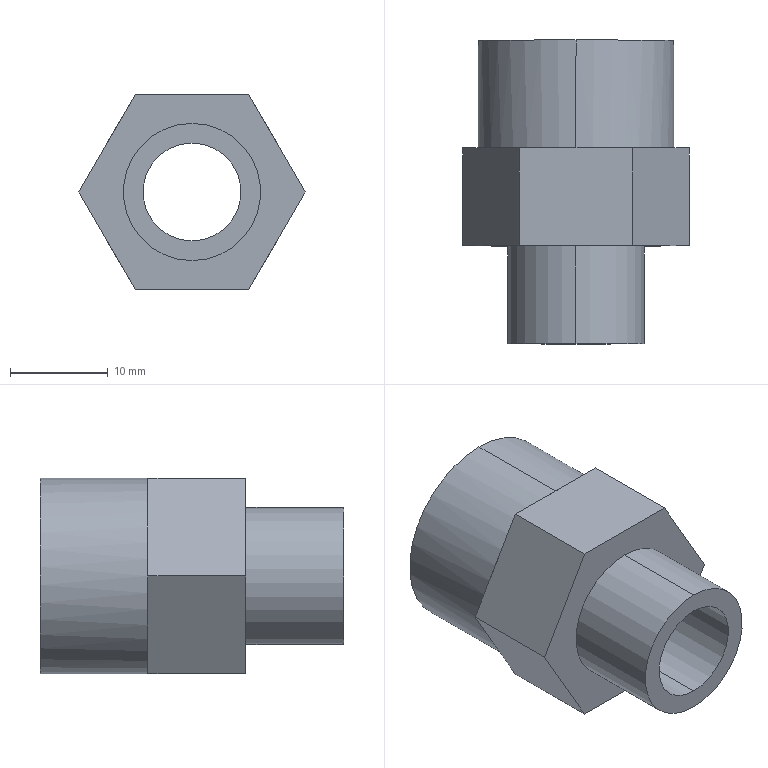Part | SolidWorks | features BossThin 1, ExtruThin 1, ICE 1 | 1 solid | 24 faces | box 23.094 x 31 x 20 mm | volume 4677 mm3 | plane 16 | cylinder 8 | commonest cylinder face diameters 10 x2 14 x2 16 x2 20 x2
STEP:
#1=CARTESIAN_POINT('',(0.,-20.,-7.));
#2=VERTEX_POINT('',#1);
#3=CARTESIAN_POINT('',(0.,-20.,7.));
#4=VERTEX_POINT('',#3);
#5=CARTESIAN_POINT('',(0.,-20.,0.));
#6=DIRECTION('',(0.,-1.,0.));
#7=DIRECTION('',(1.,0.,0.));
#8=AXIS2_PLACEMENT_3D('',#5,#6,#7);
#9=CIRCLE('',#8,7.);
#10=EDGE_CURVE('',#2,#4,#9,.T.);
#11=ORIENTED_EDGE('',*,*,#10,.F.);
#12=CARTESIAN_POINT('',(0.,-10.,-7.));
#13=VERTEX_POINT('',#12);
#14=CARTESIAN_POINT('',(0.,-20.,-7.));
#15=DIRECTION('',(0.,1.,0.));
#16=VECTOR('',#15,1000.);
#17=LINE('',#14,#16);
#18=EDGE_CURVE('',#2,#13,#17,.T.);
#19=ORIENTED_EDGE('',*,*,#18,.T.);
#20=CARTESIAN_POINT('',(0.,-10.,7.));
#21=VERTEX_POINT('',#20);
#22=CARTESIAN_POINT('',(0.,-10.,0.));
#23=DIRECTION('',(0.,-1.,0.));
#24=DIRECTION('',(1.,0.,0.));
#25=AXIS2_PLACEMENT_3D('',#22,#23,#24);
#26=CIRCLE('',#25,7.);
#27=EDGE_CURVE('',#13,#21,#26,.T.);
#28=ORIENTED_EDGE('',*,*,#27,.T.);
#29=CARTESIAN_POINT('',(0.,-20.,7.));
#30=DIRECTION('',(0.,1.,0.));
#31=VECTOR('',#30,1000.);
#32=LINE('',#29,#31);
#33=EDGE_CURVE('',#4,#21,#32,.T.);
#34=ORIENTED_EDGE('',*,*,#33,.F.);
#35=EDGE_LOOP('',(#11,#19,#28,#34));
#36=FACE_OUTER_BOUND('',#35,.T.);
#37=CARTESIAN_POINT('',(0.,-20.,0.));
#38=DIRECTION('',(0.,1.,0.));
#39=DIRECTION('',(0.,0.,1.));
#40=AXIS2_PLACEMENT_3D('',#37,#38,#39);
#41=CYLINDRICAL_SURFACE('',#40,7.);
#42=ADVANCED_FACE('',(#36),#41,.T.);
#43=CARTESIAN_POINT('',(0.,-20.,5.));
#44=VERTEX_POINT('',#43);
#45=CARTESIAN_POINT('',(0.,-20.,-5.));
#46=VERTEX_POINT('',#45);
#47=CARTESIAN_POINT('',(0.,-20.,0.));
#48=DIRECTION('',(0.,-1.,0.));
#49=DIRECTION('',(0.,0.,-1.));
#50=AXIS2_PLACEMENT_3D('',#47,#48,#49);
#51=CIRCLE('',#50,5.);
#52=EDGE_CURVE('',#44,#46,#51,.T.);
#53=ORIENTED_EDGE('',*,*,#52,.T.);
#54=CARTESIAN_POINT('',(0.,0.,-5.));
#55=VERTEX_POINT('',#54);
#56=CARTESIAN_POINT('',(0.,-10.,-5.));
#57=DIRECTION('',(0.,1.,0.));
#58=VECTOR('',#57,1000.);
#59=LINE('',#56,#58);
#60=EDGE_CURVE('',#46,#55,#59,.T.);
#61=ORIENTED_EDGE('',*,*,#60,.T.);
#62=CARTESIAN_POINT('',(0.,0.,5.));
#63=VERTEX_POINT('',#62);
#64=CARTESIAN_POINT('',(0.,0.,0.));
#65=DIRECTION('',(0.,-1.,0.));
#66=DIRECTION('',(0.,0.,-1.));
#67=AXIS2_PLACEMENT_3D('',#64,#65,#66);
#68=CIRCLE('',#67,5.);
#69=EDGE_CURVE('',#63,#55,#68,.T.);
#70=ORIENTED_EDGE('',*,*,#69,.F.);
#71=CARTESIAN_POINT('',(0.,-10.,5.));
#72=DIRECTION('',(0.,1.,0.));
#73=VECTOR('',#72,1000.);
#74=LINE('',#71,#73);
#75=EDGE_CURVE('',#44,#63,#74,.T.);
#76=ORIENTED_EDGE('',*,*,#75,.F.);
#77=EDGE_LOOP('',(#53,#61,#70,#76));
#78=FACE_OUTER_BOUND('',#77,.T.);
#79=CARTESIAN_POINT('',(0.,-10.,0.));
#80=DIRECTION('',(0.,1.,0.));
#81=DIRECTION('',(0.,0.,1.));
#82=AXIS2_PLACEMENT_3D('',#79,#80,#81);
#83=CYLINDRICAL_SURFACE('',#82,5.);
#84=ADVANCED_FACE('',(#78),#83,.F.);
#85=CARTESIAN_POINT('',(0.,11.,-8.));
#86=VERTEX_POINT('',#85);
#87=CARTESIAN_POINT('',(0.,11.,8.));
#88=VERTEX_POINT('',#87);
#89=CARTESIAN_POINT('',(0.,11.,0.));
#90=DIRECTION('',(0.,1.,0.));
#91=DIRECTION('',(1.,0.,0.));
#92=AXIS2_PLACEMENT_3D('',#89,#90,#91);
#93=CIRCLE('',#92,8.);
#94=EDGE_CURVE('',#86,#88,#93,.T.);
#95=ORIENTED_EDGE('',*,*,#94,.T.);
#96=CARTESIAN_POINT('',(0.,0.,8.));
#97=VERTEX_POINT('',#96);
#98=CARTESIAN_POINT('',(0.,11.,8.));
#99=DIRECTION('',(0.,-1.,0.));
#100=VECTOR('',#99,1000.);
#101=LINE('',#98,#100);
#102=EDGE_CURVE('',#88,#97,#101,.T.);
#103=ORIENTED_EDGE('',*,*,#102,.T.);
#104=CARTESIAN_POINT('',(0.,0.,-8.));
#105=VERTEX_POINT('',#104);
#106=CARTESIAN_POINT('',(0.,0.,0.));
#107=DIRECTION('',(0.,1.,0.));
#108=DIRECTION('',(1.,0.,0.));
#109=AXIS2_PLACEMENT_3D('',#106,#107,#108);
#110=CIRCLE('',#109,8.);
#111=EDGE_CURVE('',#105,#97,#110,.T.);
#112=ORIENTED_EDGE('',*,*,#111,.F.);
#113=CARTESIAN_POINT('',(0.,11.,-8.));
#114=DIRECTION('',(0.,-1.,0.));
#115=VECTOR('',#114,1000.);
#116=LINE('',#113,#115);
#117=EDGE_CURVE('',#86,#105,#116,.T.);
#118=ORIENTED_EDGE('',*,*,#117,.F.);
#119=EDGE_LOOP('',(#95,#103,#112,#118));
#120=FACE_OUTER_BOUND('',#119,.T.);
#121=CARTESIAN_POINT('',(0.,11.,0.));
#122=DIRECTION('',(0.,-1.,0.));
#123=DIRECTION('',(0.,0.,-1.));
#124=AXIS2_PLACEMENT_3D('',#121,#122,#123);
#125=CYLINDRICAL_SURFACE('',#124,8.);
#126=ADVANCED_FACE('',(#120),#125,.F.);
#127=CARTESIAN_POINT('',(0.,11.,10.));
#128=VERTEX_POINT('',#127);
#129=CARTESIAN_POINT('',(0.,11.,-10.));
#130=VERTEX_POINT('',#129);
#131=CARTESIAN_POINT('',(0.,11.,0.));
#132=DIRECTION('',(0.,1.,0.));
#133=DIRECTION('',(0.,0.,1.));
#134=AXIS2_PLACEMENT_3D('',#131,#132,#133);
#135=CIRCLE('',#134,10.);
#136=EDGE_CURVE('',#128,#130,#135,.T.);
#137=ORIENTED_EDGE('',*,*,#136,.F.);
#138=CARTESIAN_POINT('',(0.,0.,10.));
#139=VERTEX_POINT('',#138);
#140=CARTESIAN_POINT('',(0.,11.,10.));
#141=DIRECTION('',(0.,-1.,0.));
#142=VECTOR('',#141,1000.);
#143=LINE('',#140,#142);
#144=EDGE_CURVE('',#128,#139,#143,.T.);
#145=ORIENTED_EDGE('',*,*,#144,.T.);
#146=CARTESIAN_POINT('',(8.66,0.,5.));
#147=VERTEX_POINT('',#146);
#148=CARTESIAN_POINT('',(0.,0.,0.));
#149=DIRECTION('',(0.,1.,0.));
#150=DIRECTION('',(0.,0.,1.));
#151=AXIS2_PLACEMENT_3D('',#148,#149,#150);
#152=CIRCLE('',#151,10.);
#153=EDGE_CURVE('',#139,#147,#152,.T.);
#154=ORIENTED_EDGE('',*,*,#153,.T.);
#155=CARTESIAN_POINT('',(8.66,0.,-5.));
#156=VERTEX_POINT('',#155);
#157=CARTESIAN_POINT('',(0.,0.,0.));
#158=DIRECTION('',(0.,1.,0.));
#159=DIRECTION('',(0.,0.,1.));
#160=AXIS2_PLACEMENT_3D('',#157,#158,#159);
#161=CIRCLE('',#160,10.);
#162=EDGE_CURVE('',#147,#156,#161,.T.);
#163=ORIENTED_EDGE('',*,*,#162,.T.);
#164=CARTESIAN_POINT('',(0.,0.,-10.));
#165=VERTEX_POINT('',#164);
#166=CARTESIAN_POINT('',(0.,0.,0.));
#167=DIRECTION('',(0.,1.,0.));
#168=DIRECTION('',(0.,0.,1.));
#169=AXIS2_PLACEMENT_3D('',#166,#167,#168);
#170=CIRCLE('',#169,10.);
#171=EDGE_CURVE('',#156,#165,#170,.T.);
#172=ORIENTED_EDGE('',*,*,#171,.T.);
#173=CARTESIAN_POINT('',(0.,11.,-10.));
#174=DIRECTION('',(0.,-1.,0.));
#175=VECTOR('',#174,1000.);
#176=LINE('',#173,#175);
#177=EDGE_CURVE('',#130,#165,#176,.T.);
#178=ORIENTED_EDGE('',*,*,#177,.F.);
#179=EDGE_LOOP('',(#137,#145,#154,#163,#172,#178));
#180=FACE_OUTER_BOUND('',#179,.T.);
#181=CARTESIAN_POINT('',(0.,11.,0.));
#182=DIRECTION('',(0.,-1.,0.));
#183=DIRECTION('',(0.,0.,-1.));
#184=AXIS2_PLACEMENT_3D('',#181,#182,#183);
#185=CYLINDRICAL_SURFACE('',#184,10.);
#186=ADVANCED_FACE('',(#180),#185,.T.);
#187=CARTESIAN_POINT('',(5.774,-10.,-10.));
#188=VERTEX_POINT('',#187);
#189=CARTESIAN_POINT('',(11.547,-10.,0.));
#190=VERTEX_POINT('',#189);
#191=CARTESIAN_POINT('',(5.774,-10.,-10.));
#192=DIRECTION('',(0.5,0.,0.866));
#193=VECTOR('',#192,1000.);
#194=LINE('',#191,#193);
#195=EDGE_CURVE('',#188,#190,#194,.T.);
#196=ORIENTED_EDGE('',*,*,#195,.T.);
#197=CARTESIAN_POINT('',(5.774,-10.,10.));
#198=VERTEX_POINT('',#197);
#199=CARTESIAN_POINT('',(11.547,-10.,0.));
#200=DIRECTION('',(-0.5,0.,0.866));
#201=VECTOR('',#200,1000.);
#202=LINE('',#199,#201);
#203=EDGE_CURVE('',#190,#198,#202,.T.);
#204=ORIENTED_EDGE('',*,*,#203,.T.);
#205=CARTESIAN_POINT('',(-5.774,-10.,10.));
#206=VERTEX_POINT('',#205);
#207=CARTESIAN_POINT('',(5.774,-10.,10.));
#208=DIRECTION('',(-1.,0.,0.));
#209=VECTOR('',#208,1000.);
#210=LINE('',#207,#209);
#211=EDGE_CURVE('',#198,#206,#210,.T.);
#212=ORIENTED_EDGE('',*,*,#211,.T.);
#213=CARTESIAN_POINT('',(-11.547,-10.,0.));
#214=VERTEX_POINT('',#213);
#215=CARTESIAN_POINT('',(-5.774,-10.,10.));
#216=DIRECTION('',(-0.5,0.,-0.866));
#217=VECTOR('',#216,1000.);
#218=LINE('',#215,#217);
#219=EDGE_CURVE('',#206,#214,#218,.T.);
#220=ORIENTED_EDGE('',*,*,#219,.T.);
#221=CARTESIAN_POINT('',(-5.774,-10.,-10.));
#222=VERTEX_POINT('',#221);
#223=CARTESIAN_POINT('',(-11.547,-10.,0.));
#224=DIRECTION('',(0.5,0.,-0.866));
#225=VECTOR('',#224,1000.);
#226=LINE('',#223,#225);
#227=EDGE_CURVE('',#214,#222,#226,.T.);
#228=ORIENTED_EDGE('',*,*,#227,.T.);
#229=CARTESIAN_POINT('',(-5.774,-10.,-10.));
#230=DIRECTION('',(1.,0.,0.));
#231=VECTOR('',#230,1000.);
#232=LINE('',#229,#231);
#233=EDGE_CURVE('',#222,#188,#232,.T.);
#234=ORIENTED_EDGE('',*,*,#233,.T.);
#235=EDGE_LOOP('',(#196,#204,#212,#220,#228,#234));
#236=FACE_OUTER_BOUND('',#235,.T.);
#237=CARTESIAN_POINT('',(0.,-10.,0.));
#238=DIRECTION('',(0.,-1.,0.));
#239=DIRECTION('',(1.,0.,0.));
#240=AXIS2_PLACEMENT_3D('',#237,#238,#239);
#241=CIRCLE('',#240,7.);
#242=EDGE_CURVE('',#21,#13,#241,.T.);
#243=ORIENTED_EDGE('',*,*,#242,.F.);
#244=ORIENTED_EDGE('',*,*,#27,.F.);
#245=EDGE_LOOP('',(#243,#244));
#246=FACE_BOUND('',#245,.T.);
#247=CARTESIAN_POINT('',(0.,-10.,0.));
#248=DIRECTION('',(0.,-1.,0.));
#249=DIRECTION('',(0.,0.,-1.));
#250=AXIS2_PLACEMENT_3D('',#247,#248,#249);
#251=PLANE('',#250);
#252=ADVANCED_FACE('',(#236,#246),#251,.T.);
#253=CARTESIAN_POINT('',(0.,11.,0.));
#254=DIRECTION('',(0.,1.,0.));
#255=DIRECTION('',(0.,0.,1.));
#256=AXIS2_PLACEMENT_3D('',#253,#254,#255);
#257=CIRCLE('',#256,10.);
#258=EDGE_CURVE('',#130,#128,#257,.T.);
#259=ORIENTED_EDGE('',*,*,#258,.T.);
#260=ORIENTED_EDGE('',*,*,#136,.T.);
#261=EDGE_LOOP('',(#259,#260));
#262=FACE_OUTER_BOUND('',#261,.T.);
#263=ORIENTED_EDGE('',*,*,#94,.F.);
#264=CARTESIAN_POINT('',(0.,11.,0.));
#265=DIRECTION('',(0.,1.,0.));
#266=DIRECTION('',(1.,0.,0.));
#267=AXIS2_PLACEMENT_3D('',#264,#265,#266);
#268=CIRCLE('',#267,8.);
#269=EDGE_CURVE('',#88,#86,#268,.T.);
#270=ORIENTED_EDGE('',*,*,#269,.F.);
#271=EDGE_LOOP('',(#263,#270));
#272=FACE_BOUND('',#271,.T.);
#273=CARTESIAN_POINT('',(0.,11.,0.));
#274=DIRECTION('',(0.,1.,0.));
#275=DIRECTION('',(0.,0.,1.));
#276=AXIS2_PLACEMENT_3D('',#273,#274,#275);
#277=PLANE('',#276);
#278=ADVANCED_FACE('',(#262,#272),#277,.T.);
#279=ORIENTED_EDGE('',*,*,#144,.F.);
#280=ORIENTED_EDGE('',*,*,#258,.F.);
#281=ORIENTED_EDGE('',*,*,#177,.T.);
#282=CARTESIAN_POINT('',(-8.66,0.,-5.));
#283=VERTEX_POINT('',#282);
#284=CARTESIAN_POINT('',(0.,0.,0.));
#285=DIRECTION('',(0.,1.,0.));
#286=DIRECTION('',(0.,0.,1.));
#287=AXIS2_PLACEMENT_3D('',#284,#285,#286);
#288=CIRCLE('',#287,10.);
#289=EDGE_CURVE('',#165,#283,#288,.T.);
#290=ORIENTED_EDGE('',*,*,#289,.T.);
#291=CARTESIAN_POINT('',(-8.66,0.,5.));
#292=VERTEX_POINT('',#291);
#293=CARTESIAN_POINT('',(0.,0.,0.));
#294=DIRECTION('',(0.,1.,0.));
#295=DIRECTION('',(0.,0.,1.));
#296=AXIS2_PLACEMENT_3D('',#293,#294,#295);
#297=CIRCLE('',#296,10.);
#298=EDGE_CURVE('',#283,#292,#297,.T.);
#299=ORIENTED_EDGE('',*,*,#298,.T.);
#300=CARTESIAN_POINT('',(0.,0.,0.));
#301=DIRECTION('',(0.,1.,0.));
#302=DIRECTION('',(0.,0.,1.));
#303=AXIS2_PLACEMENT_3D('',#300,#301,#302);
#304=CIRCLE('',#303,10.);
#305=EDGE_CURVE('',#292,#139,#304,.T.);
#306=ORIENTED_EDGE('',*,*,#305,.T.);
#307=EDGE_LOOP('',(#279,#280,#281,#290,#299,#306));
#308=FACE_OUTER_BOUND('',#307,.T.);
#309=CARTESIAN_POINT('',(0.,11.,0.));
#310=DIRECTION('',(0.,-1.,0.));
#311=DIRECTION('',(0.,0.,-1.));
#312=AXIS2_PLACEMENT_3D('',#309,#310,#311);
#313=CYLINDRICAL_SURFACE('',#312,10.);
#314=ADVANCED_FACE('',(#308),#313,.T.);
#315=ORIENTED_EDGE('',*,*,#102,.F.);
#316=ORIENTED_EDGE('',*,*,#269,.T.);
#317=ORIENTED_EDGE('',*,*,#117,.T.);
#318=CARTESIAN_POINT('',(0.,0.,0.));
#319=DIRECTION('',(0.,1.,0.));
#320=DIRECTION('',(1.,0.,0.));
#321=AXIS2_PLACEMENT_3D('',#318,#319,#320);
#322=CIRCLE('',#321,8.);
#323=EDGE_CURVE('',#97,#105,#322,.T.);
#324=ORIENTED_EDGE('',*,*,#323,.F.);
#325=EDGE_LOOP('',(#315,#316,#317,#324));
#326=FACE_OUTER_BOUND('',#325,.T.);
#327=CARTESIAN_POINT('',(0.,11.,0.));
#328=DIRECTION('',(0.,-1.,0.));
#329=DIRECTION('',(0.,0.,-1.));
#330=AXIS2_PLACEMENT_3D('',#327,#328,#329);
#331=CYLINDRICAL_SURFACE('',#330,8.);
#332=ADVANCED_FACE('',(#326),#331,.F.);
#333=ORIENTED_EDGE('',*,*,#153,.F.);
#334=CARTESIAN_POINT('',(5.774,0.,10.));
#335=VERTEX_POINT('',#334);
#336=CARTESIAN_POINT('',(5.774,0.,10.));
#337=DIRECTION('',(-1.,0.,0.));
#338=VECTOR('',#337,1000.);
#339=LINE('',#336,#338);
#340=EDGE_CURVE('',#335,#139,#339,.T.);
#341=ORIENTED_EDGE('',*,*,#340,.F.);
#342=CARTESIAN_POINT('',(11.547,0.,0.));
#343=DIRECTION('',(-0.5,0.,0.866));
#344=VECTOR('',#343,1000.);
#345=LINE('',#342,#344);
#346=EDGE_CURVE('',#147,#335,#345,.T.);
#347=ORIENTED_EDGE('',*,*,#346,.F.);
#348=EDGE_LOOP('',(#333,#341,#347));
#349=FACE_OUTER_BOUND('',#348,.T.);
#350=CARTESIAN_POINT('',(0.,0.,0.));
#351=DIRECTION('',(0.,-1.,0.));
#352=DIRECTION('',(0.,0.,-1.));
#353=AXIS2_PLACEMENT_3D('',#350,#351,#352);
#354=PLANE('',#353);
#355=ADVANCED_FACE('',(#349),#354,.F.);
#356=ORIENTED_EDGE('',*,*,#162,.F.);
#357=CARTESIAN_POINT('',(11.547,0.,0.));
#358=VERTEX_POINT('',#357);
#359=CARTESIAN_POINT('',(11.547,0.,0.));
#360=DIRECTION('',(-0.5,0.,0.866));
#361=VECTOR('',#360,1000.);
#362=LINE('',#359,#361);
#363=EDGE_CURVE('',#358,#147,#362,.T.);
#364=ORIENTED_EDGE('',*,*,#363,.F.);
#365=CARTESIAN_POINT('',(5.774,0.,-10.));
#366=DIRECTION('',(0.5,0.,0.866));
#367=VECTOR('',#366,1000.);
#368=LINE('',#365,#367);
#369=EDGE_CURVE('',#156,#358,#368,.T.);
#370=ORIENTED_EDGE('',*,*,#369,.F.);
#371=EDGE_LOOP('',(#356,#364,#370));
#372=FACE_OUTER_BOUND('',#371,.T.);
#373=CARTESIAN_POINT('',(0.,0.,0.));
#374=DIRECTION('',(0.,-1.,0.));
#375=DIRECTION('',(0.,0.,-1.));
#376=AXIS2_PLACEMENT_3D('',#373,#374,#375);
#377=PLANE('',#376);
#378=ADVANCED_FACE('',(#372),#377,.F.);
#379=ORIENTED_EDGE('',*,*,#171,.F.);
#380=CARTESIAN_POINT('',(5.774,0.,-10.));
#381=VERTEX_POINT('',#380);
#382=CARTESIAN_POINT('',(5.774,0.,-10.));
#383=DIRECTION('',(0.5,0.,0.866));
#384=VECTOR('',#383,1000.);
#385=LINE('',#382,#384);
#386=EDGE_CURVE('',#381,#156,#385,.T.);
#387=ORIENTED_EDGE('',*,*,#386,.F.);
#388=CARTESIAN_POINT('',(-5.774,0.,-10.));
#389=DIRECTION('',(1.,0.,0.));
#390=VECTOR('',#389,1000.);
#391=LINE('',#388,#390);
#392=EDGE_CURVE('',#165,#381,#391,.T.);
#393=ORIENTED_EDGE('',*,*,#392,.F.);
#394=EDGE_LOOP('',(#379,#387,#393));
#395=FACE_OUTER_BOUND('',#394,.T.);
#396=CARTESIAN_POINT('',(0.,0.,0.));
#397=DIRECTION('',(0.,-1.,0.));
#398=DIRECTION('',(0.,0.,-1.));
#399=AXIS2_PLACEMENT_3D('',#396,#397,#398);
#400=PLANE('',#399);
#401=ADVANCED_FACE('',(#395),#400,.F.);
#402=ORIENTED_EDGE('',*,*,#289,.F.);
#403=CARTESIAN_POINT('',(-5.774,0.,-10.));
#404=VERTEX_POINT('',#403);
#405=CARTESIAN_POINT('',(-5.774,0.,-10.));
#406=DIRECTION('',(1.,0.,0.));
#407=VECTOR('',#406,1000.);
#408=LINE('',#405,#407);
#409=EDGE_CURVE('',#404,#165,#408,.T.);
#410=ORIENTED_EDGE('',*,*,#409,.F.);
#411=CARTESIAN_POINT('',(-11.547,0.,0.));
#412=DIRECTION('',(0.5,0.,-0.866));
#413=VECTOR('',#412,1000.);
#414=LINE('',#411,#413);
#415=EDGE_CURVE('',#283,#404,#414,.T.);
#416=ORIENTED_EDGE('',*,*,#415,.F.);
#417=EDGE_LOOP('',(#402,#410,#416));
#418=FACE_OUTER_BOUND('',#417,.T.);
#419=CARTESIAN_POINT('',(0.,0.,0.));
#420=DIRECTION('',(0.,-1.,0.));
#421=DIRECTION('',(0.,0.,-1.));
#422=AXIS2_PLACEMENT_3D('',#419,#420,#421);
#423=PLANE('',#422);
#424=ADVANCED_FACE('',(#418),#423,.F.);
#425=ORIENTED_EDGE('',*,*,#298,.F.);
#426=CARTESIAN_POINT('',(-11.547,0.,0.));
#427=VERTEX_POINT('',#426);
#428=CARTESIAN_POINT('',(-11.547,0.,0.));
#429=DIRECTION('',(0.5,0.,-0.866));
#430=VECTOR('',#429,1000.);
#431=LINE('',#428,#430);
#432=EDGE_CURVE('',#427,#283,#431,.T.);
#433=ORIENTED_EDGE('',*,*,#432,.F.);
#434=CARTESIAN_POINT('',(-5.774,0.,10.));
#435=DIRECTION('',(-0.5,0.,-0.866));
#436=VECTOR('',#435,1000.);
#437=LINE('',#434,#436);
#438=EDGE_CURVE('',#292,#427,#437,.T.);
#439=ORIENTED_EDGE('',*,*,#438,.F.);
#440=EDGE_LOOP('',(#425,#433,#439));
#441=FACE_OUTER_BOUND('',#440,.T.);
#442=CARTESIAN_POINT('',(0.,0.,0.));
#443=DIRECTION('',(0.,-1.,0.));
#444=DIRECTION('',(0.,0.,-1.));
#445=AXIS2_PLACEMENT_3D('',#442,#443,#444);
#446=PLANE('',#445);
#447=ADVANCED_FACE('',(#441),#446,.F.);
#448=ORIENTED_EDGE('',*,*,#69,.T.);
#449=CARTESIAN_POINT('',(0.,0.,0.));
#450=DIRECTION('',(0.,-1.,0.));
#451=DIRECTION('',(0.,0.,-1.));
#452=AXIS2_PLACEMENT_3D('',#449,#450,#451);
#453=CIRCLE('',#452,5.);
#454=EDGE_CURVE('',#55,#63,#453,.T.);
#455=ORIENTED_EDGE('',*,*,#454,.T.);
#456=EDGE_LOOP('',(#448,#455));
#457=FACE_BOUND('',#456,.T.);
#458=ORIENTED_EDGE('',*,*,#111,.T.);
#459=ORIENTED_EDGE('',*,*,#323,.T.);
#460=EDGE_LOOP('',(#458,#459));
#461=FACE_OUTER_BOUND('',#460,.T.);
#462=CARTESIAN_POINT('',(0.,0.,0.));
#463=DIRECTION('',(0.,-1.,0.));
#464=DIRECTION('',(0.,0.,-1.));
#465=AXIS2_PLACEMENT_3D('',#462,#463,#464);
#466=PLANE('',#465);
#467=ADVANCED_FACE('',(#457,#461),#466,.F.);
#468=ORIENTED_EDGE('',*,*,#305,.F.);
#469=CARTESIAN_POINT('',(-5.774,0.,10.));
#470=VERTEX_POINT('',#469);
#471=CARTESIAN_POINT('',(-5.774,0.,10.));
#472=DIRECTION('',(-0.5,0.,-0.866));
#473=VECTOR('',#472,1000.);
#474=LINE('',#471,#473);
#475=EDGE_CURVE('',#470,#292,#474,.T.);
#476=ORIENTED_EDGE('',*,*,#475,.F.);
#477=CARTESIAN_POINT('',(5.774,0.,10.));
#478=DIRECTION('',(-1.,0.,0.));
#479=VECTOR('',#478,1000.);
#480=LINE('',#477,#479);
#481=EDGE_CURVE('',#139,#470,#480,.T.);
#482=ORIENTED_EDGE('',*,*,#481,.F.);
#483=EDGE_LOOP('',(#468,#476,#482));
#484=FACE_OUTER_BOUND('',#483,.T.);
#485=CARTESIAN_POINT('',(0.,0.,0.));
#486=DIRECTION('',(0.,-1.,0.));
#487=DIRECTION('',(0.,0.,-1.));
#488=AXIS2_PLACEMENT_3D('',#485,#486,#487);
#489=PLANE('',#488);
#490=ADVANCED_FACE('',(#484),#489,.F.);
#491=ORIENTED_EDGE('',*,*,#386,.T.);
#492=ORIENTED_EDGE('',*,*,#369,.T.);
#493=CARTESIAN_POINT('',(11.547,-10.,0.));
#494=DIRECTION('',(0.,1.,0.));
#495=VECTOR('',#494,1000.);
#496=LINE('',#493,#495);
#497=EDGE_CURVE('',#190,#358,#496,.T.);
#498=ORIENTED_EDGE('',*,*,#497,.F.);
#499=ORIENTED_EDGE('',*,*,#195,.F.);
#500=CARTESIAN_POINT('',(5.774,-10.,-10.));
#501=DIRECTION('',(0.,1.,0.));
#502=VECTOR('',#501,1000.);
#503=LINE('',#500,#502);
#504=EDGE_CURVE('',#188,#381,#503,.T.);
#505=ORIENTED_EDGE('',*,*,#504,.T.);
#506=EDGE_LOOP('',(#491,#492,#498,#499,#505));
#507=FACE_OUTER_BOUND('',#506,.T.);
#508=CARTESIAN_POINT('',(5.774,-10.,-10.));
#509=DIRECTION('',(-0.866,0.,0.5));
#510=DIRECTION('',(0.5,0.,0.866));
#511=AXIS2_PLACEMENT_3D('',#508,#509,#510);
#512=PLANE('',#511);
#513=ADVANCED_FACE('',(#507),#512,.F.);
#514=ORIENTED_EDGE('',*,*,#363,.T.);
#515=ORIENTED_EDGE('',*,*,#346,.T.);
#516=CARTESIAN_POINT('',(5.774,-10.,10.));
#517=DIRECTION('',(0.,1.,0.));
#518=VECTOR('',#517,1000.);
#519=LINE('',#516,#518);
#520=EDGE_CURVE('',#198,#335,#519,.T.);
#521=ORIENTED_EDGE('',*,*,#520,.F.);
#522=ORIENTED_EDGE('',*,*,#203,.F.);
#523=ORIENTED_EDGE('',*,*,#497,.T.);
#524=EDGE_LOOP('',(#514,#515,#521,#522,#523));
#525=FACE_OUTER_BOUND('',#524,.T.);
#526=CARTESIAN_POINT('',(11.547,-10.,0.));
#527=DIRECTION('',(-0.866,0.,-0.5));
#528=DIRECTION('',(-0.5,0.,0.866));
#529=AXIS2_PLACEMENT_3D('',#526,#527,#528);
#530=PLANE('',#529);
#531=ADVANCED_FACE('',(#525),#530,.F.);
#532=ORIENTED_EDGE('',*,*,#340,.T.);
#533=ORIENTED_EDGE('',*,*,#481,.T.);
#534=CARTESIAN_POINT('',(-5.774,-10.,10.));
#535=DIRECTION('',(0.,1.,0.));
#536=VECTOR('',#535,1000.);
#537=LINE('',#534,#536);
#538=EDGE_CURVE('',#206,#470,#537,.T.);
#539=ORIENTED_EDGE('',*,*,#538,.F.);
#540=ORIENTED_EDGE('',*,*,#211,.F.);
#541=ORIENTED_EDGE('',*,*,#520,.T.);
#542=EDGE_LOOP('',(#532,#533,#539,#540,#541));
#543=FACE_OUTER_BOUND('',#542,.T.);
#544=CARTESIAN_POINT('',(5.774,-10.,10.));
#545=DIRECTION('',(0.,0.,-1.));
#546=DIRECTION('',(-1.,0.,0.));
#547=AXIS2_PLACEMENT_3D('',#544,#545,#546);
#548=PLANE('',#547);
#549=ADVANCED_FACE('',(#543),#548,.F.);
#550=ORIENTED_EDGE('',*,*,#475,.T.);
#551=ORIENTED_EDGE('',*,*,#438,.T.);
#552=CARTESIAN_POINT('',(-11.547,-10.,0.));
#553=DIRECTION('',(0.,1.,0.));
#554=VECTOR('',#553,1000.);
#555=LINE('',#552,#554);
#556=EDGE_CURVE('',#214,#427,#555,.T.);
#557=ORIENTED_EDGE('',*,*,#556,.F.);
#558=ORIENTED_EDGE('',*,*,#219,.F.);
#559=ORIENTED_EDGE('',*,*,#538,.T.);
#560=EDGE_LOOP('',(#550,#551,#557,#558,#559));
#561=FACE_OUTER_BOUND('',#560,.T.);
#562=CARTESIAN_POINT('',(-5.774,-10.,10.));
#563=DIRECTION('',(0.866,0.,-0.5));
#564=DIRECTION('',(-0.5,0.,-0.866));
#565=AXIS2_PLACEMENT_3D('',#562,#563,#564);
#566=PLANE('',#565);
#567=ADVANCED_FACE('',(#561),#566,.F.);
#568=ORIENTED_EDGE('',*,*,#432,.T.);
#569=ORIENTED_EDGE('',*,*,#415,.T.);
#570=CARTESIAN_POINT('',(-5.774,-10.,-10.));
#571=DIRECTION('',(0.,1.,0.));
#572=VECTOR('',#571,1000.);
#573=LINE('',#570,#572);
#574=EDGE_CURVE('',#222,#404,#573,.T.);
#575=ORIENTED_EDGE('',*,*,#574,.F.);
#576=ORIENTED_EDGE('',*,*,#227,.F.);
#577=ORIENTED_EDGE('',*,*,#556,.T.);
#578=EDGE_LOOP('',(#568,#569,#575,#576,#577));
#579=FACE_OUTER_BOUND('',#578,.T.);
#580=CARTESIAN_POINT('',(-11.547,-10.,0.));
#581=DIRECTION('',(0.866,0.,0.5));
#582=DIRECTION('',(0.5,0.,-0.866));
#583=AXIS2_PLACEMENT_3D('',#580,#581,#582);
#584=PLANE('',#583);
#585=ADVANCED_FACE('',(#579),#584,.F.);
#586=ORIENTED_EDGE('',*,*,#409,.T.);
#587=ORIENTED_EDGE('',*,*,#392,.T.);
#588=ORIENTED_EDGE('',*,*,#504,.F.);
#589=ORIENTED_EDGE('',*,*,#233,.F.);
#590=ORIENTED_EDGE('',*,*,#574,.T.);
#591=EDGE_LOOP('',(#586,#587,#588,#589,#590));
#592=FACE_OUTER_BOUND('',#591,.T.);
#593=CARTESIAN_POINT('',(-5.774,-10.,-10.));
#594=DIRECTION('',(0.,0.,1.));
#595=DIRECTION('',(1.,0.,0.));
#596=AXIS2_PLACEMENT_3D('',#593,#594,#595);
#597=PLANE('',#596);
#598=ADVANCED_FACE('',(#592),#597,.F.);
#599=ORIENTED_EDGE('',*,*,#60,.F.);
#600=CARTESIAN_POINT('',(0.,-20.,0.));
#601=DIRECTION('',(0.,-1.,0.));
#602=DIRECTION('',(0.,0.,-1.));
#603=AXIS2_PLACEMENT_3D('',#600,#601,#602);
#604=CIRCLE('',#603,5.);
#605=EDGE_CURVE('',#46,#44,#604,.T.);
#606=ORIENTED_EDGE('',*,*,#605,.T.);
#607=ORIENTED_EDGE('',*,*,#75,.T.);
#608=ORIENTED_EDGE('',*,*,#454,.F.);
#609=EDGE_LOOP('',(#599,#606,#607,#608));
#610=FACE_OUTER_BOUND('',#609,.T.);
#611=CARTESIAN_POINT('',(0.,-10.,0.));
#612=DIRECTION('',(0.,1.,0.));
#613=DIRECTION('',(0.,0.,1.));
#614=AXIS2_PLACEMENT_3D('',#611,#612,#613);
#615=CYLINDRICAL_SURFACE('',#614,5.);
#616=ADVANCED_FACE('',(#610),#615,.F.);
#617=CARTESIAN_POINT('',(0.,-20.,0.));
#618=DIRECTION('',(0.,-1.,0.));
#619=DIRECTION('',(1.,0.,0.));
#620=AXIS2_PLACEMENT_3D('',#617,#618,#619);
#621=CIRCLE('',#620,7.);
#622=EDGE_CURVE('',#4,#2,#621,.T.);
#623=ORIENTED_EDGE('',*,*,#622,.T.);
#624=ORIENTED_EDGE('',*,*,#10,.T.);
#625=EDGE_LOOP('',(#623,#624));
#626=FACE_OUTER_BOUND('',#625,.T.);
#627=ORIENTED_EDGE('',*,*,#52,.F.);
#628=ORIENTED_EDGE('',*,*,#605,.F.);
#629=EDGE_LOOP('',(#627,#628));
#630=FACE_BOUND('',#629,.T.);
#631=CARTESIAN_POINT('',(0.,-20.,0.));
#632=DIRECTION('',(0.,-1.,0.));
#633=DIRECTION('',(0.,0.,-1.));
#634=AXIS2_PLACEMENT_3D('',#631,#632,#633);
#635=PLANE('',#634);
#636=ADVANCED_FACE('',(#626,#630),#635,.T.);
#637=ORIENTED_EDGE('',*,*,#18,.F.);
#638=ORIENTED_EDGE('',*,*,#622,.F.);
#639=ORIENTED_EDGE('',*,*,#33,.T.);
#640=ORIENTED_EDGE('',*,*,#242,.T.);
#641=EDGE_LOOP('',(#637,#638,#639,#640));
#642=FACE_OUTER_BOUND('',#641,.T.);
#643=CARTESIAN_POINT('',(0.,-20.,0.));
#644=DIRECTION('',(0.,1.,0.));
#645=DIRECTION('',(0.,0.,1.));
#646=AXIS2_PLACEMENT_3D('',#643,#644,#645);
#647=CYLINDRICAL_SURFACE('',#646,7.);
#648=ADVANCED_FACE('',(#642),#647,.T.);
#649=CLOSED_SHELL('',(#42,#84,#126,#186,#252,#278,#314,#332,#355,#378,#401,#424,#447,#467,#490,#513,#531,#549,#567,#585,#598,#616,#636,#648));
#650=MANIFOLD_SOLID_BREP('',#649);
#651=CARTESIAN_POINT('',(0.,0.,0.));
#652=DIRECTION('',(0.,0.,1.));
#653=DIRECTION('',(1.,0.,0.));
#654=AXIS2_PLACEMENT_3D('',#651,#652,#653);
#655=(LENGTH_UNIT()NAMED_UNIT(*)SI_UNIT(.MILLI.,.METRE.));
#656=UNCERTAINTY_MEASURE_WITH_UNIT(LENGTH_MEASURE(0.00001),#655,'','');
#657=(NAMED_UNIT(*)PLANE_ANGLE_UNIT()SI_UNIT($,.RADIAN.));
#658=(NAMED_UNIT(*)SI_UNIT($,.STERADIAN.)SOLID_ANGLE_UNIT());
#659=(GEOMETRIC_REPRESENTATION_CONTEXT(3)GLOBAL_UNCERTAINTY_ASSIGNED_CONTEXT((#656))GLOBAL_UNIT_ASSIGNED_CONTEXT((#655,#657,#658))REPRESENTATION_CONTEXT('',''));
#660=ADVANCED_BREP_SHAPE_REPRESENTATION('',(#650,#654),#659);